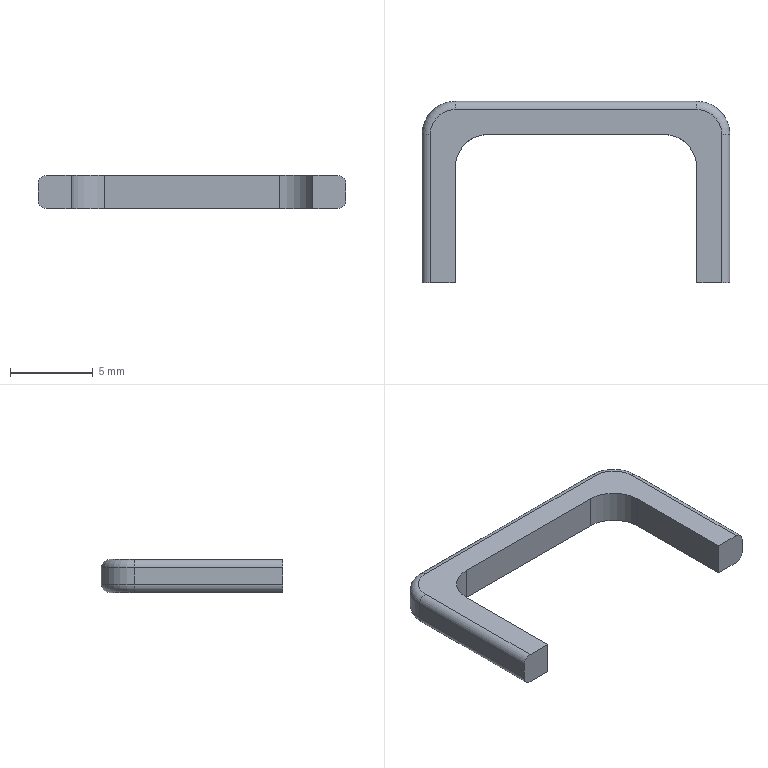Part | SolidWorks | features Fillet 2, ExtruThin 1 | 1 solid | 24 faces | box 18.597 x 10.954 x 2 mm | volume 141.898 mm3 | plane 10 | cylinder 10 | torus 4 | commonest cylinder face diameters 1 x6 4 x4
STEP:
#1=CARTESIAN_POINT('',(-2.,8.954,1.5));
#2=VERTEX_POINT('',#1);
#3=CARTESIAN_POINT('',(-2.,8.954,0.5));
#4=VERTEX_POINT('',#3);
#5=CARTESIAN_POINT('',(-2.,8.954,2.));
#6=DIRECTION('',(0.,0.,-1.));
#7=VECTOR('',#6,1000.);
#8=LINE('',#5,#7);
#9=EDGE_CURVE('',#2,#4,#8,.T.);
#10=ORIENTED_EDGE('',*,*,#9,.T.);
#11=CARTESIAN_POINT('',(-2.,0.,0.5));
#12=VERTEX_POINT('',#11);
#13=CARTESIAN_POINT('',(-2.,0.,0.5));
#14=DIRECTION('',(0.,-1.,0.));
#15=VECTOR('',#14,1000.);
#16=LINE('',#13,#15);
#17=EDGE_CURVE('',#4,#12,#16,.T.);
#18=ORIENTED_EDGE('',*,*,#17,.T.);
#19=CARTESIAN_POINT('',(-2.,0.,1.5));
#20=VERTEX_POINT('',#19);
#21=CARTESIAN_POINT('',(-2.,0.,2.));
#22=DIRECTION('',(0.,0.,-1.));
#23=VECTOR('',#22,1000.);
#24=LINE('',#21,#23);
#25=EDGE_CURVE('',#20,#12,#24,.T.);
#26=ORIENTED_EDGE('',*,*,#25,.F.);
#27=CARTESIAN_POINT('',(-2.,8.954,1.5));
#28=DIRECTION('',(0.,1.,0.));
#29=VECTOR('',#28,1000.);
#30=LINE('',#27,#29);
#31=EDGE_CURVE('',#20,#2,#30,.T.);
#32=ORIENTED_EDGE('',*,*,#31,.T.);
#33=EDGE_LOOP('',(#10,#18,#26,#32));
#34=FACE_OUTER_BOUND('',#33,.T.);
#35=CARTESIAN_POINT('',(-2.,0.,2.));
#36=DIRECTION('',(1.,0.,0.));
#37=DIRECTION('',(0.,0.,-1.));
#38=AXIS2_PLACEMENT_3D('',#35,#36,#37);
#39=PLANE('',#38);
#40=ADVANCED_FACE('',(#34),#39,.F.);
#41=ORIENTED_EDGE('',*,*,#25,.T.);
#42=CARTESIAN_POINT('',(-1.5,0.,0.));
#43=VERTEX_POINT('',#42);
#44=CARTESIAN_POINT('',(-1.5,0.,0.5));
#45=DIRECTION('',(0.,-1.,0.));
#46=DIRECTION('',(0.,0.,-1.));
#47=AXIS2_PLACEMENT_3D('',#44,#45,#46);
#48=CIRCLE('',#47,0.5);
#49=EDGE_CURVE('',#12,#43,#48,.T.);
#50=ORIENTED_EDGE('',*,*,#49,.T.);
#51=CARTESIAN_POINT('',(0.,0.,0.));
#52=VERTEX_POINT('',#51);
#53=CARTESIAN_POINT('',(0.,0.,0.));
#54=DIRECTION('',(-1.,0.,0.));
#55=VECTOR('',#54,1000.);
#56=LINE('',#53,#55);
#57=EDGE_CURVE('',#52,#43,#56,.T.);
#58=ORIENTED_EDGE('',*,*,#57,.F.);
#59=CARTESIAN_POINT('',(0.,0.,2.));
#60=VERTEX_POINT('',#59);
#61=CARTESIAN_POINT('',(0.,0.,2.));
#62=DIRECTION('',(0.,0.,-1.));
#63=VECTOR('',#62,1000.);
#64=LINE('',#61,#63);
#65=EDGE_CURVE('',#60,#52,#64,.T.);
#66=ORIENTED_EDGE('',*,*,#65,.F.);
#67=CARTESIAN_POINT('',(-1.5,0.,2.));
#68=VERTEX_POINT('',#67);
#69=CARTESIAN_POINT('',(0.,0.,2.));
#70=DIRECTION('',(-1.,0.,0.));
#71=VECTOR('',#70,1000.);
#72=LINE('',#69,#71);
#73=EDGE_CURVE('',#60,#68,#72,.T.);
#74=ORIENTED_EDGE('',*,*,#73,.T.);
#75=CARTESIAN_POINT('',(-1.5,0.,1.5));
#76=DIRECTION('',(0.,-1.,0.));
#77=DIRECTION('',(0.,0.,-1.));
#78=AXIS2_PLACEMENT_3D('',#75,#76,#77);
#79=CIRCLE('',#78,0.5);
#80=EDGE_CURVE('',#68,#20,#79,.T.);
#81=ORIENTED_EDGE('',*,*,#80,.T.);
#82=EDGE_LOOP('',(#41,#50,#58,#66,#74,#81));
#83=FACE_OUTER_BOUND('',#82,.T.);
#84=CARTESIAN_POINT('',(0.,0.,2.));
#85=DIRECTION('',(0.,-1.,0.));
#86=DIRECTION('',(0.,0.,-1.));
#87=AXIS2_PLACEMENT_3D('',#84,#85,#86);
#88=PLANE('',#87);
#89=ADVANCED_FACE('',(#83),#88,.T.);
#90=CARTESIAN_POINT('',(0.,6.954,0.));
#91=VERTEX_POINT('',#90);
#92=CARTESIAN_POINT('',(0.,0.,0.));
#93=DIRECTION('',(0.,-1.,0.));
#94=VECTOR('',#93,1000.);
#95=LINE('',#92,#94);
#96=EDGE_CURVE('',#91,#52,#95,.T.);
#97=ORIENTED_EDGE('',*,*,#96,.F.);
#98=CARTESIAN_POINT('',(0.,6.954,2.));
#99=VERTEX_POINT('',#98);
#100=CARTESIAN_POINT('',(0.,6.954,2.));
#101=DIRECTION('',(0.,0.,1.));
#102=VECTOR('',#101,1000.);
#103=LINE('',#100,#102);
#104=EDGE_CURVE('',#91,#99,#103,.T.);
#105=ORIENTED_EDGE('',*,*,#104,.T.);
#106=CARTESIAN_POINT('',(0.,0.,2.));
#107=DIRECTION('',(0.,-1.,0.));
#108=VECTOR('',#107,1000.);
#109=LINE('',#106,#108);
#110=EDGE_CURVE('',#99,#60,#109,.T.);
#111=ORIENTED_EDGE('',*,*,#110,.T.);
#112=ORIENTED_EDGE('',*,*,#65,.T.);
#113=EDGE_LOOP('',(#97,#105,#111,#112));
#114=FACE_OUTER_BOUND('',#113,.T.);
#115=CARTESIAN_POINT('',(0.,0.,2.));
#116=DIRECTION('',(1.,0.,0.));
#117=DIRECTION('',(0.,0.,-1.));
#118=AXIS2_PLACEMENT_3D('',#115,#116,#117);
#119=PLANE('',#118);
#120=ADVANCED_FACE('',(#114),#119,.T.);
#121=CARTESIAN_POINT('',(12.597,8.954,0.));
#122=VERTEX_POINT('',#121);
#123=CARTESIAN_POINT('',(2.,8.954,0.));
#124=VERTEX_POINT('',#123);
#125=CARTESIAN_POINT('',(0.,8.954,0.));
#126=DIRECTION('',(-1.,0.,0.));
#127=VECTOR('',#126,1000.);
#128=LINE('',#125,#127);
#129=EDGE_CURVE('',#122,#124,#128,.T.);
#130=ORIENTED_EDGE('',*,*,#129,.F.);
#131=CARTESIAN_POINT('',(12.597,8.954,2.));
#132=VERTEX_POINT('',#131);
#133=CARTESIAN_POINT('',(12.597,8.954,2.));
#134=DIRECTION('',(0.,0.,1.));
#135=VECTOR('',#134,1000.);
#136=LINE('',#133,#135);
#137=EDGE_CURVE('',#122,#132,#136,.T.);
#138=ORIENTED_EDGE('',*,*,#137,.T.);
#139=CARTESIAN_POINT('',(2.,8.954,2.));
#140=VERTEX_POINT('',#139);
#141=CARTESIAN_POINT('',(0.,8.954,2.));
#142=DIRECTION('',(-1.,0.,0.));
#143=VECTOR('',#142,1000.);
#144=LINE('',#141,#143);
#145=EDGE_CURVE('',#132,#140,#144,.T.);
#146=ORIENTED_EDGE('',*,*,#145,.T.);
#147=CARTESIAN_POINT('',(2.,8.954,0.));
#148=DIRECTION('',(0.,0.,-1.));
#149=VECTOR('',#148,1000.);
#150=LINE('',#147,#149);
#151=EDGE_CURVE('',#140,#124,#150,.T.);
#152=ORIENTED_EDGE('',*,*,#151,.T.);
#153=EDGE_LOOP('',(#130,#138,#146,#152));
#154=FACE_OUTER_BOUND('',#153,.T.);
#155=CARTESIAN_POINT('',(0.,8.954,2.));
#156=DIRECTION('',(0.,-1.,0.));
#157=DIRECTION('',(0.,0.,-1.));
#158=AXIS2_PLACEMENT_3D('',#155,#156,#157);
#159=PLANE('',#158);
#160=ADVANCED_FACE('',(#154),#159,.T.);
#161=CARTESIAN_POINT('',(14.597,0.,2.));
#162=VERTEX_POINT('',#161);
#163=CARTESIAN_POINT('',(14.597,6.954,2.));
#164=VERTEX_POINT('',#163);
#165=CARTESIAN_POINT('',(14.597,0.,2.));
#166=DIRECTION('',(0.,1.,0.));
#167=VECTOR('',#166,1000.);
#168=LINE('',#165,#167);
#169=EDGE_CURVE('',#162,#164,#168,.T.);
#170=ORIENTED_EDGE('',*,*,#169,.T.);
#171=CARTESIAN_POINT('',(14.597,6.954,0.));
#172=VERTEX_POINT('',#171);
#173=CARTESIAN_POINT('',(14.597,6.954,0.));
#174=DIRECTION('',(0.,0.,-1.));
#175=VECTOR('',#174,1000.);
#176=LINE('',#173,#175);
#177=EDGE_CURVE('',#164,#172,#176,.T.);
#178=ORIENTED_EDGE('',*,*,#177,.T.);
#179=CARTESIAN_POINT('',(14.597,0.,0.));
#180=VERTEX_POINT('',#179);
#181=CARTESIAN_POINT('',(14.597,0.,0.));
#182=DIRECTION('',(0.,1.,0.));
#183=VECTOR('',#182,1000.);
#184=LINE('',#181,#183);
#185=EDGE_CURVE('',#180,#172,#184,.T.);
#186=ORIENTED_EDGE('',*,*,#185,.F.);
#187=CARTESIAN_POINT('',(14.597,0.,2.));
#188=DIRECTION('',(0.,0.,-1.));
#189=VECTOR('',#188,1000.);
#190=LINE('',#187,#189);
#191=EDGE_CURVE('',#162,#180,#190,.T.);
#192=ORIENTED_EDGE('',*,*,#191,.F.);
#193=EDGE_LOOP('',(#170,#178,#186,#192));
#194=FACE_OUTER_BOUND('',#193,.T.);
#195=CARTESIAN_POINT('',(14.597,0.,2.));
#196=DIRECTION('',(-1.,0.,0.));
#197=DIRECTION('',(0.,0.,1.));
#198=AXIS2_PLACEMENT_3D('',#195,#196,#197);
#199=PLANE('',#198);
#200=ADVANCED_FACE('',(#194),#199,.T.);
#201=CARTESIAN_POINT('',(16.097,0.,0.));
#202=VERTEX_POINT('',#201);
#203=CARTESIAN_POINT('',(16.597,0.,0.));
#204=DIRECTION('',(-1.,0.,0.));
#205=VECTOR('',#204,1000.);
#206=LINE('',#203,#205);
#207=EDGE_CURVE('',#202,#180,#206,.T.);
#208=ORIENTED_EDGE('',*,*,#207,.F.);
#209=CARTESIAN_POINT('',(16.597,0.,0.5));
#210=VERTEX_POINT('',#209);
#211=CARTESIAN_POINT('',(16.097,0.,0.5));
#212=DIRECTION('',(0.,-1.,0.));
#213=DIRECTION('',(0.,0.,-1.));
#214=AXIS2_PLACEMENT_3D('',#211,#212,#213);
#215=CIRCLE('',#214,0.5);
#216=EDGE_CURVE('',#202,#210,#215,.T.);
#217=ORIENTED_EDGE('',*,*,#216,.T.);
#218=CARTESIAN_POINT('',(16.597,0.,1.5));
#219=VERTEX_POINT('',#218);
#220=CARTESIAN_POINT('',(16.597,0.,2.));
#221=DIRECTION('',(0.,0.,-1.));
#222=VECTOR('',#221,1000.);
#223=LINE('',#220,#222);
#224=EDGE_CURVE('',#219,#210,#223,.T.);
#225=ORIENTED_EDGE('',*,*,#224,.F.);
#226=CARTESIAN_POINT('',(16.097,0.,2.));
#227=VERTEX_POINT('',#226);
#228=CARTESIAN_POINT('',(16.097,0.,1.5));
#229=DIRECTION('',(0.,-1.,0.));
#230=DIRECTION('',(0.,0.,-1.));
#231=AXIS2_PLACEMENT_3D('',#228,#229,#230);
#232=CIRCLE('',#231,0.5);
#233=EDGE_CURVE('',#219,#227,#232,.T.);
#234=ORIENTED_EDGE('',*,*,#233,.T.);
#235=CARTESIAN_POINT('',(16.597,0.,2.));
#236=DIRECTION('',(-1.,0.,0.));
#237=VECTOR('',#236,1000.);
#238=LINE('',#235,#237);
#239=EDGE_CURVE('',#227,#162,#238,.T.);
#240=ORIENTED_EDGE('',*,*,#239,.T.);
#241=ORIENTED_EDGE('',*,*,#191,.T.);
#242=EDGE_LOOP('',(#208,#217,#225,#234,#240,#241));
#243=FACE_OUTER_BOUND('',#242,.T.);
#244=CARTESIAN_POINT('',(16.597,0.,2.));
#245=DIRECTION('',(0.,-1.,0.));
#246=DIRECTION('',(0.,0.,-1.));
#247=AXIS2_PLACEMENT_3D('',#244,#245,#246);
#248=PLANE('',#247);
#249=ADVANCED_FACE('',(#243),#248,.T.);
#250=ORIENTED_EDGE('',*,*,#224,.T.);
#251=CARTESIAN_POINT('',(16.597,8.954,0.5));
#252=VERTEX_POINT('',#251);
#253=CARTESIAN_POINT('',(16.597,0.,0.5));
#254=DIRECTION('',(0.,1.,0.));
#255=VECTOR('',#254,1000.);
#256=LINE('',#253,#255);
#257=EDGE_CURVE('',#210,#252,#256,.T.);
#258=ORIENTED_EDGE('',*,*,#257,.T.);
#259=CARTESIAN_POINT('',(16.597,8.954,1.5));
#260=VERTEX_POINT('',#259);
#261=CARTESIAN_POINT('',(16.597,8.954,2.));
#262=DIRECTION('',(0.,0.,1.));
#263=VECTOR('',#262,1000.);
#264=LINE('',#261,#263);
#265=EDGE_CURVE('',#252,#260,#264,.T.);
#266=ORIENTED_EDGE('',*,*,#265,.T.);
#267=CARTESIAN_POINT('',(16.597,0.,1.5));
#268=DIRECTION('',(0.,-1.,0.));
#269=VECTOR('',#268,1000.);
#270=LINE('',#267,#269);
#271=EDGE_CURVE('',#260,#219,#270,.T.);
#272=ORIENTED_EDGE('',*,*,#271,.T.);
#273=EDGE_LOOP('',(#250,#258,#266,#272));
#274=FACE_OUTER_BOUND('',#273,.T.);
#275=CARTESIAN_POINT('',(16.597,0.,2.));
#276=DIRECTION('',(-1.,0.,0.));
#277=DIRECTION('',(0.,0.,1.));
#278=AXIS2_PLACEMENT_3D('',#275,#276,#277);
#279=PLANE('',#278);
#280=ADVANCED_FACE('',(#274),#279,.F.);
#281=CARTESIAN_POINT('',(14.597,10.954,1.5));
#282=VERTEX_POINT('',#281);
#283=CARTESIAN_POINT('',(14.597,10.954,0.5));
#284=VERTEX_POINT('',#283);
#285=CARTESIAN_POINT('',(14.597,10.954,2.));
#286=DIRECTION('',(0.,0.,-1.));
#287=VECTOR('',#286,1000.);
#288=LINE('',#285,#287);
#289=EDGE_CURVE('',#282,#284,#288,.T.);
#290=ORIENTED_EDGE('',*,*,#289,.T.);
#291=CARTESIAN_POINT('',(0.,10.954,0.5));
#292=VERTEX_POINT('',#291);
#293=CARTESIAN_POINT('',(0.,10.954,0.5));
#294=DIRECTION('',(-1.,0.,0.));
#295=VECTOR('',#294,1000.);
#296=LINE('',#293,#295);
#297=EDGE_CURVE('',#284,#292,#296,.T.);
#298=ORIENTED_EDGE('',*,*,#297,.T.);
#299=CARTESIAN_POINT('',(0.,10.954,1.5));
#300=VERTEX_POINT('',#299);
#301=CARTESIAN_POINT('',(0.,10.954,2.));
#302=DIRECTION('',(0.,0.,1.));
#303=VECTOR('',#302,1000.);
#304=LINE('',#301,#303);
#305=EDGE_CURVE('',#292,#300,#304,.T.);
#306=ORIENTED_EDGE('',*,*,#305,.T.);
#307=CARTESIAN_POINT('',(14.597,10.954,1.5));
#308=DIRECTION('',(1.,0.,0.));
#309=VECTOR('',#308,1000.);
#310=LINE('',#307,#309);
#311=EDGE_CURVE('',#300,#282,#310,.T.);
#312=ORIENTED_EDGE('',*,*,#311,.T.);
#313=EDGE_LOOP('',(#290,#298,#306,#312));
#314=FACE_OUTER_BOUND('',#313,.T.);
#315=CARTESIAN_POINT('',(0.,10.954,2.));
#316=DIRECTION('',(0.,-1.,0.));
#317=DIRECTION('',(0.,0.,-1.));
#318=AXIS2_PLACEMENT_3D('',#315,#316,#317);
#319=PLANE('',#318);
#320=ADVANCED_FACE('',(#314),#319,.F.);
#321=ORIENTED_EDGE('',*,*,#239,.F.);
#322=CARTESIAN_POINT('',(16.097,8.954,2.));
#323=VERTEX_POINT('',#322);
#324=CARTESIAN_POINT('',(16.097,8.954,2.));
#325=DIRECTION('',(0.,1.,0.));
#326=VECTOR('',#325,1000.);
#327=LINE('',#324,#326);
#328=EDGE_CURVE('',#227,#323,#327,.T.);
#329=ORIENTED_EDGE('',*,*,#328,.T.);
#330=CARTESIAN_POINT('',(14.597,10.454,2.));
#331=VERTEX_POINT('',#330);
#332=CARTESIAN_POINT('',(14.597,8.954,2.));
#333=DIRECTION('',(0.,0.,1.));
#334=DIRECTION('',(1.,0.,0.));
#335=AXIS2_PLACEMENT_3D('',#332,#333,#334);
#336=CIRCLE('',#335,1.5);
#337=EDGE_CURVE('',#323,#331,#336,.T.);
#338=ORIENTED_EDGE('',*,*,#337,.T.);
#339=CARTESIAN_POINT('',(0.,10.454,2.));
#340=VERTEX_POINT('',#339);
#341=CARTESIAN_POINT('',(0.,10.454,2.));
#342=DIRECTION('',(-1.,0.,0.));
#343=VECTOR('',#342,1000.);
#344=LINE('',#341,#343);
#345=EDGE_CURVE('',#331,#340,#344,.T.);
#346=ORIENTED_EDGE('',*,*,#345,.T.);
#347=CARTESIAN_POINT('',(-1.5,8.954,2.));
#348=VERTEX_POINT('',#347);
#349=CARTESIAN_POINT('',(0.,8.954,2.));
#350=DIRECTION('',(0.,0.,1.));
#351=DIRECTION('',(1.,0.,0.));
#352=AXIS2_PLACEMENT_3D('',#349,#350,#351);
#353=CIRCLE('',#352,1.5);
#354=EDGE_CURVE('',#340,#348,#353,.T.);
#355=ORIENTED_EDGE('',*,*,#354,.T.);
#356=CARTESIAN_POINT('',(-1.5,0.,2.));
#357=DIRECTION('',(0.,-1.,0.));
#358=VECTOR('',#357,1000.);
#359=LINE('',#356,#358);
#360=EDGE_CURVE('',#348,#68,#359,.T.);
#361=ORIENTED_EDGE('',*,*,#360,.T.);
#362=ORIENTED_EDGE('',*,*,#73,.F.);
#363=ORIENTED_EDGE('',*,*,#110,.F.);
#364=CARTESIAN_POINT('',(2.,6.954,2.));
#365=DIRECTION('',(0.,0.,-1.));
#366=DIRECTION('',(1.,0.,0.));
#367=AXIS2_PLACEMENT_3D('',#364,#365,#366);
#368=CIRCLE('',#367,2.);
#369=EDGE_CURVE('',#99,#140,#368,.T.);
#370=ORIENTED_EDGE('',*,*,#369,.T.);
#371=ORIENTED_EDGE('',*,*,#145,.F.);
#372=CARTESIAN_POINT('',(12.597,6.954,2.));
#373=DIRECTION('',(0.,0.,-1.));
#374=DIRECTION('',(1.,0.,0.));
#375=AXIS2_PLACEMENT_3D('',#372,#373,#374);
#376=CIRCLE('',#375,2.);
#377=EDGE_CURVE('',#132,#164,#376,.T.);
#378=ORIENTED_EDGE('',*,*,#377,.T.);
#379=ORIENTED_EDGE('',*,*,#169,.F.);
#380=EDGE_LOOP('',(#321,#329,#338,#346,#355,#361,#362,#363,#370,#371,#378,#379));
#381=FACE_OUTER_BOUND('',#380,.T.);
#382=CARTESIAN_POINT('',(0.,0.,2.));
#383=DIRECTION('',(0.,0.,1.));
#384=DIRECTION('',(1.,0.,0.));
#385=AXIS2_PLACEMENT_3D('',#382,#383,#384);
#386=PLANE('',#385);
#387=ADVANCED_FACE('',(#381),#386,.T.);
#388=CARTESIAN_POINT('',(14.597,10.454,0.));
#389=VERTEX_POINT('',#388);
#390=CARTESIAN_POINT('',(16.097,8.954,0.));
#391=VERTEX_POINT('',#390);
#392=CARTESIAN_POINT('',(14.597,8.954,0.));
#393=DIRECTION('',(0.,0.,-1.));
#394=DIRECTION('',(1.,0.,0.));
#395=AXIS2_PLACEMENT_3D('',#392,#393,#394);
#396=CIRCLE('',#395,1.5);
#397=EDGE_CURVE('',#389,#391,#396,.T.);
#398=ORIENTED_EDGE('',*,*,#397,.T.);
#399=CARTESIAN_POINT('',(16.097,0.,0.));
#400=DIRECTION('',(0.,-1.,0.));
#401=VECTOR('',#400,1000.);
#402=LINE('',#399,#401);
#403=EDGE_CURVE('',#391,#202,#402,.T.);
#404=ORIENTED_EDGE('',*,*,#403,.T.);
#405=ORIENTED_EDGE('',*,*,#207,.T.);
#406=ORIENTED_EDGE('',*,*,#185,.T.);
#407=CARTESIAN_POINT('',(12.597,6.954,0.));
#408=DIRECTION('',(0.,0.,1.));
#409=DIRECTION('',(1.,0.,0.));
#410=AXIS2_PLACEMENT_3D('',#407,#408,#409);
#411=CIRCLE('',#410,2.);
#412=EDGE_CURVE('',#172,#122,#411,.T.);
#413=ORIENTED_EDGE('',*,*,#412,.T.);
#414=ORIENTED_EDGE('',*,*,#129,.T.);
#415=CARTESIAN_POINT('',(2.,6.954,0.));
#416=DIRECTION('',(0.,0.,1.));
#417=DIRECTION('',(1.,0.,0.));
#418=AXIS2_PLACEMENT_3D('',#415,#416,#417);
#419=CIRCLE('',#418,2.);
#420=EDGE_CURVE('',#124,#91,#419,.T.);
#421=ORIENTED_EDGE('',*,*,#420,.T.);
#422=ORIENTED_EDGE('',*,*,#96,.T.);
#423=ORIENTED_EDGE('',*,*,#57,.T.);
#424=CARTESIAN_POINT('',(-1.5,8.954,0.));
#425=VERTEX_POINT('',#424);
#426=CARTESIAN_POINT('',(-1.5,0.,0.));
#427=DIRECTION('',(0.,1.,0.));
#428=VECTOR('',#427,1000.);
#429=LINE('',#426,#428);
#430=EDGE_CURVE('',#43,#425,#429,.T.);
#431=ORIENTED_EDGE('',*,*,#430,.T.);
#432=CARTESIAN_POINT('',(0.,10.454,0.));
#433=VERTEX_POINT('',#432);
#434=CARTESIAN_POINT('',(0.,8.954,0.));
#435=DIRECTION('',(0.,0.,-1.));
#436=DIRECTION('',(1.,0.,0.));
#437=AXIS2_PLACEMENT_3D('',#434,#435,#436);
#438=CIRCLE('',#437,1.5);
#439=EDGE_CURVE('',#425,#433,#438,.T.);
#440=ORIENTED_EDGE('',*,*,#439,.T.);
#441=CARTESIAN_POINT('',(0.,10.454,0.));
#442=DIRECTION('',(1.,0.,0.));
#443=VECTOR('',#442,1000.);
#444=LINE('',#441,#443);
#445=EDGE_CURVE('',#433,#389,#444,.T.);
#446=ORIENTED_EDGE('',*,*,#445,.T.);
#447=EDGE_LOOP('',(#398,#404,#405,#406,#413,#414,#421,#422,#423,#431,#440,#446));
#448=FACE_OUTER_BOUND('',#447,.T.);
#449=CARTESIAN_POINT('',(0.,0.,0.));
#450=DIRECTION('',(0.,0.,1.));
#451=DIRECTION('',(1.,0.,0.));
#452=AXIS2_PLACEMENT_3D('',#449,#450,#451);
#453=PLANE('',#452);
#454=ADVANCED_FACE('',(#448),#453,.F.);
#455=ORIENTED_EDGE('',*,*,#377,.F.);
#456=ORIENTED_EDGE('',*,*,#137,.F.);
#457=ORIENTED_EDGE('',*,*,#412,.F.);
#458=ORIENTED_EDGE('',*,*,#177,.F.);
#459=EDGE_LOOP('',(#455,#456,#457,#458));
#460=FACE_OUTER_BOUND('',#459,.T.);
#461=CARTESIAN_POINT('',(12.597,6.954,2.));
#462=DIRECTION('',(0.,0.,1.));
#463=DIRECTION('',(1.,0.,0.));
#464=AXIS2_PLACEMENT_3D('',#461,#462,#463);
#465=CYLINDRICAL_SURFACE('',#464,2.);
#466=ADVANCED_FACE('',(#460),#465,.F.);
#467=ORIENTED_EDGE('',*,*,#369,.F.);
#468=ORIENTED_EDGE('',*,*,#104,.F.);
#469=ORIENTED_EDGE('',*,*,#420,.F.);
#470=ORIENTED_EDGE('',*,*,#151,.F.);
#471=EDGE_LOOP('',(#467,#468,#469,#470));
#472=FACE_OUTER_BOUND('',#471,.T.);
#473=CARTESIAN_POINT('',(2.,6.954,2.));
#474=DIRECTION('',(0.,0.,1.));
#475=DIRECTION('',(1.,0.,0.));
#476=AXIS2_PLACEMENT_3D('',#473,#474,#475);
#477=CYLINDRICAL_SURFACE('',#476,2.);
#478=ADVANCED_FACE('',(#472),#477,.F.);
#479=ORIENTED_EDGE('',*,*,#265,.F.);
#480=CARTESIAN_POINT('',(14.597,8.954,0.5));
#481=DIRECTION('',(0.,0.,1.));
#482=DIRECTION('',(1.,0.,0.));
#483=AXIS2_PLACEMENT_3D('',#480,#481,#482);
#484=CIRCLE('',#483,2.);
#485=EDGE_CURVE('',#252,#284,#484,.T.);
#486=ORIENTED_EDGE('',*,*,#485,.T.);
#487=ORIENTED_EDGE('',*,*,#289,.F.);
#488=CARTESIAN_POINT('',(14.597,8.954,1.5));
#489=DIRECTION('',(0.,0.,-1.));
#490=DIRECTION('',(1.,0.,0.));
#491=AXIS2_PLACEMENT_3D('',#488,#489,#490);
#492=CIRCLE('',#491,2.);
#493=EDGE_CURVE('',#282,#260,#492,.T.);
#494=ORIENTED_EDGE('',*,*,#493,.T.);
#495=EDGE_LOOP('',(#479,#486,#487,#494));
#496=FACE_OUTER_BOUND('',#495,.T.);
#497=CARTESIAN_POINT('',(14.597,8.954,2.));
#498=DIRECTION('',(0.,0.,-1.));
#499=DIRECTION('',(-1.,0.,0.));
#500=AXIS2_PLACEMENT_3D('',#497,#498,#499);
#501=CYLINDRICAL_SURFACE('',#500,2.);
#502=ADVANCED_FACE('',(#496),#501,.T.);
#503=ORIENTED_EDGE('',*,*,#305,.F.);
#504=CARTESIAN_POINT('',(0.,8.954,0.5));
#505=DIRECTION('',(0.,0.,1.));
#506=DIRECTION('',(1.,0.,0.));
#507=AXIS2_PLACEMENT_3D('',#504,#505,#506);
#508=CIRCLE('',#507,2.);
#509=EDGE_CURVE('',#292,#4,#508,.T.);
#510=ORIENTED_EDGE('',*,*,#509,.T.);
#511=ORIENTED_EDGE('',*,*,#9,.F.);
#512=CARTESIAN_POINT('',(0.,8.954,1.5));
#513=DIRECTION('',(0.,0.,-1.));
#514=DIRECTION('',(1.,0.,0.));
#515=AXIS2_PLACEMENT_3D('',#512,#513,#514);
#516=CIRCLE('',#515,2.);
#517=EDGE_CURVE('',#2,#300,#516,.T.);
#518=ORIENTED_EDGE('',*,*,#517,.T.);
#519=EDGE_LOOP('',(#503,#510,#511,#518));
#520=FACE_OUTER_BOUND('',#519,.T.);
#521=CARTESIAN_POINT('',(0.,8.954,2.));
#522=DIRECTION('',(0.,0.,-1.));
#523=DIRECTION('',(-1.,0.,0.));
#524=AXIS2_PLACEMENT_3D('',#521,#522,#523);
#525=CYLINDRICAL_SURFACE('',#524,2.);
#526=ADVANCED_FACE('',(#520),#525,.T.);
#527=ORIENTED_EDGE('',*,*,#49,.F.);
#528=ORIENTED_EDGE('',*,*,#17,.F.);
#529=CARTESIAN_POINT('',(-1.5,8.954,0.5));
#530=DIRECTION('',(0.,1.,0.));
#531=DIRECTION('',(0.,0.,1.));
#532=AXIS2_PLACEMENT_3D('',#529,#530,#531);
#533=CIRCLE('',#532,0.5);
#534=EDGE_CURVE('',#425,#4,#533,.T.);
#535=ORIENTED_EDGE('',*,*,#534,.F.);
#536=ORIENTED_EDGE('',*,*,#430,.F.);
#537=EDGE_LOOP('',(#527,#528,#535,#536));
#538=FACE_OUTER_BOUND('',#537,.T.);
#539=CARTESIAN_POINT('',(-1.5,0.,0.5));
#540=DIRECTION('',(0.,-1.,0.));
#541=DIRECTION('',(0.,0.,-1.));
#542=AXIS2_PLACEMENT_3D('',#539,#540,#541);
#543=CYLINDRICAL_SURFACE('',#542,0.5);
#544=ADVANCED_FACE('',(#538),#543,.T.);
#545=ORIENTED_EDGE('',*,*,#534,.T.);
#546=ORIENTED_EDGE('',*,*,#509,.F.);
#547=CARTESIAN_POINT('',(0.,10.454,0.5));
#548=DIRECTION('',(1.,0.,0.));
#549=DIRECTION('',(0.,0.,-1.));
#550=AXIS2_PLACEMENT_3D('',#547,#548,#549);
#551=CIRCLE('',#550,0.5);
#552=EDGE_CURVE('',#433,#292,#551,.T.);
#553=ORIENTED_EDGE('',*,*,#552,.F.);
#554=ORIENTED_EDGE('',*,*,#439,.F.);
#555=EDGE_LOOP('',(#545,#546,#553,#554));
#556=FACE_OUTER_BOUND('',#555,.T.);
#557=CARTESIAN_POINT('',(0.,8.954,0.5));
#558=DIRECTION('',(0.,0.,1.));
#559=DIRECTION('',(1.,0.,0.));
#560=AXIS2_PLACEMENT_3D('',#557,#558,#559);
#561=TOROIDAL_SURFACE('',#560,1.5,0.5);
#562=ADVANCED_FACE('',(#556),#561,.T.);
#563=ORIENTED_EDGE('',*,*,#552,.T.);
#564=ORIENTED_EDGE('',*,*,#297,.F.);
#565=CARTESIAN_POINT('',(14.597,10.454,0.5));
#566=DIRECTION('',(1.,0.,0.));
#567=DIRECTION('',(0.,0.,-1.));
#568=AXIS2_PLACEMENT_3D('',#565,#566,#567);
#569=CIRCLE('',#568,0.5);
#570=EDGE_CURVE('',#389,#284,#569,.T.);
#571=ORIENTED_EDGE('',*,*,#570,.F.);
#572=ORIENTED_EDGE('',*,*,#445,.F.);
#573=EDGE_LOOP('',(#563,#564,#571,#572));
#574=FACE_OUTER_BOUND('',#573,.T.);
#575=CARTESIAN_POINT('',(0.,10.454,0.5));
#576=DIRECTION('',(-1.,0.,0.));
#577=DIRECTION('',(0.,0.,1.));
#578=AXIS2_PLACEMENT_3D('',#575,#576,#577);
#579=CYLINDRICAL_SURFACE('',#578,0.5);
#580=ADVANCED_FACE('',(#574),#579,.T.);
#581=ORIENTED_EDGE('',*,*,#570,.T.);
#582=ORIENTED_EDGE('',*,*,#485,.F.);
#583=CARTESIAN_POINT('',(16.097,8.954,0.5));
#584=DIRECTION('',(0.,-1.,0.));
#585=DIRECTION('',(0.,0.,-1.));
#586=AXIS2_PLACEMENT_3D('',#583,#584,#585);
#587=CIRCLE('',#586,0.5);
#588=EDGE_CURVE('',#391,#252,#587,.T.);
#589=ORIENTED_EDGE('',*,*,#588,.F.);
#590=ORIENTED_EDGE('',*,*,#397,.F.);
#591=EDGE_LOOP('',(#581,#582,#589,#590));
#592=FACE_OUTER_BOUND('',#591,.T.);
#593=CARTESIAN_POINT('',(14.597,8.954,0.5));
#594=DIRECTION('',(0.,0.,1.));
#595=DIRECTION('',(1.,0.,0.));
#596=AXIS2_PLACEMENT_3D('',#593,#594,#595);
#597=TOROIDAL_SURFACE('',#596,1.5,0.5);
#598=ADVANCED_FACE('',(#592),#597,.T.);
#599=ORIENTED_EDGE('',*,*,#216,.F.);
#600=ORIENTED_EDGE('',*,*,#403,.F.);
#601=ORIENTED_EDGE('',*,*,#588,.T.);
#602=ORIENTED_EDGE('',*,*,#257,.F.);
#603=EDGE_LOOP('',(#599,#600,#601,#602));
#604=FACE_OUTER_BOUND('',#603,.T.);
#605=CARTESIAN_POINT('',(16.097,0.,0.5));
#606=DIRECTION('',(0.,1.,0.));
#607=DIRECTION('',(0.,0.,1.));
#608=AXIS2_PLACEMENT_3D('',#605,#606,#607);
#609=CYLINDRICAL_SURFACE('',#608,0.5);
#610=ADVANCED_FACE('',(#604),#609,.T.);
#611=ORIENTED_EDGE('',*,*,#80,.F.);
#612=ORIENTED_EDGE('',*,*,#360,.F.);
#613=CARTESIAN_POINT('',(-1.5,8.954,1.5));
#614=DIRECTION('',(0.,1.,0.));
#615=DIRECTION('',(0.,0.,1.));
#616=AXIS2_PLACEMENT_3D('',#613,#614,#615);
#617=CIRCLE('',#616,0.5);
#618=EDGE_CURVE('',#2,#348,#617,.T.);
#619=ORIENTED_EDGE('',*,*,#618,.F.);
#620=ORIENTED_EDGE('',*,*,#31,.F.);
#621=EDGE_LOOP('',(#611,#612,#619,#620));
#622=FACE_OUTER_BOUND('',#621,.T.);
#623=CARTESIAN_POINT('',(-1.5,0.,1.5));
#624=DIRECTION('',(0.,1.,0.));
#625=DIRECTION('',(0.,0.,1.));
#626=AXIS2_PLACEMENT_3D('',#623,#624,#625);
#627=CYLINDRICAL_SURFACE('',#626,0.5);
#628=ADVANCED_FACE('',(#622),#627,.T.);
#629=ORIENTED_EDGE('',*,*,#618,.T.);
#630=ORIENTED_EDGE('',*,*,#354,.F.);
#631=CARTESIAN_POINT('',(0.,10.454,1.5));
#632=DIRECTION('',(1.,0.,0.));
#633=DIRECTION('',(0.,0.,-1.));
#634=AXIS2_PLACEMENT_3D('',#631,#632,#633);
#635=CIRCLE('',#634,0.5);
#636=EDGE_CURVE('',#300,#340,#635,.T.);
#637=ORIENTED_EDGE('',*,*,#636,.F.);
#638=ORIENTED_EDGE('',*,*,#517,.F.);
#639=EDGE_LOOP('',(#629,#630,#637,#638));
#640=FACE_OUTER_BOUND('',#639,.T.);
#641=CARTESIAN_POINT('',(0.,8.954,1.5));
#642=DIRECTION('',(0.,0.,1.));
#643=DIRECTION('',(1.,0.,0.));
#644=AXIS2_PLACEMENT_3D('',#641,#642,#643);
#645=TOROIDAL_SURFACE('',#644,1.5,0.5);
#646=ADVANCED_FACE('',(#640),#645,.T.);
#647=ORIENTED_EDGE('',*,*,#636,.T.);
#648=ORIENTED_EDGE('',*,*,#345,.F.);
#649=CARTESIAN_POINT('',(14.597,10.454,1.5));
#650=DIRECTION('',(1.,0.,0.));
#651=DIRECTION('',(0.,0.,-1.));
#652=AXIS2_PLACEMENT_3D('',#649,#650,#651);
#653=CIRCLE('',#652,0.5);
#654=EDGE_CURVE('',#282,#331,#653,.T.);
#655=ORIENTED_EDGE('',*,*,#654,.F.);
#656=ORIENTED_EDGE('',*,*,#311,.F.);
#657=EDGE_LOOP('',(#647,#648,#655,#656));
#658=FACE_OUTER_BOUND('',#657,.T.);
#659=CARTESIAN_POINT('',(0.,10.454,1.5));
#660=DIRECTION('',(1.,0.,0.));
#661=DIRECTION('',(0.,0.,-1.));
#662=AXIS2_PLACEMENT_3D('',#659,#660,#661);
#663=CYLINDRICAL_SURFACE('',#662,0.5);
#664=ADVANCED_FACE('',(#658),#663,.T.);
#665=ORIENTED_EDGE('',*,*,#654,.T.);
#666=ORIENTED_EDGE('',*,*,#337,.F.);
#667=CARTESIAN_POINT('',(16.097,8.954,1.5));
#668=DIRECTION('',(0.,-1.,0.));
#669=DIRECTION('',(0.,0.,-1.));
#670=AXIS2_PLACEMENT_3D('',#667,#668,#669);
#671=CIRCLE('',#670,0.5);
#672=EDGE_CURVE('',#260,#323,#671,.T.);
#673=ORIENTED_EDGE('',*,*,#672,.F.);
#674=ORIENTED_EDGE('',*,*,#493,.F.);
#675=EDGE_LOOP('',(#665,#666,#673,#674));
#676=FACE_OUTER_BOUND('',#675,.T.);
#677=CARTESIAN_POINT('',(14.597,8.954,1.5));
#678=DIRECTION('',(0.,0.,1.));
#679=DIRECTION('',(1.,0.,0.));
#680=AXIS2_PLACEMENT_3D('',#677,#678,#679);
#681=TOROIDAL_SURFACE('',#680,1.5,0.5);
#682=ADVANCED_FACE('',(#676),#681,.T.);
#683=ORIENTED_EDGE('',*,*,#233,.F.);
#684=ORIENTED_EDGE('',*,*,#271,.F.);
#685=ORIENTED_EDGE('',*,*,#672,.T.);
#686=ORIENTED_EDGE('',*,*,#328,.F.);
#687=EDGE_LOOP('',(#683,#684,#685,#686));
#688=FACE_OUTER_BOUND('',#687,.T.);
#689=CARTESIAN_POINT('',(16.097,0.,1.5));
#690=DIRECTION('',(0.,-1.,0.));
#691=DIRECTION('',(0.,0.,-1.));
#692=AXIS2_PLACEMENT_3D('',#689,#690,#691);
#693=CYLINDRICAL_SURFACE('',#692,0.5);
#694=ADVANCED_FACE('',(#688),#693,.T.);
#695=CLOSED_SHELL('',(#40,#89,#120,#160,#200,#249,#280,#320,#387,#454,#466,#478,#502,#526,#544,#562,#580,#598,#610,#628,#646,#664,#682,#694));
#696=MANIFOLD_SOLID_BREP('',#695);
#697=CARTESIAN_POINT('',(0.,0.,0.));
#698=DIRECTION('',(0.,0.,1.));
#699=DIRECTION('',(1.,0.,0.));
#700=AXIS2_PLACEMENT_3D('',#697,#698,#699);
#701=(LENGTH_UNIT()NAMED_UNIT(*)SI_UNIT(.MILLI.,.METRE.));
#702=UNCERTAINTY_MEASURE_WITH_UNIT(LENGTH_MEASURE(0.00001),#701,'','');
#703=(NAMED_UNIT(*)PLANE_ANGLE_UNIT()SI_UNIT($,.RADIAN.));
#704=(NAMED_UNIT(*)SI_UNIT($,.STERADIAN.)SOLID_ANGLE_UNIT());
#705=(GEOMETRIC_REPRESENTATION_CONTEXT(3)GLOBAL_UNCERTAINTY_ASSIGNED_CONTEXT((#702))GLOBAL_UNIT_ASSIGNED_CONTEXT((#701,#703,#704))REPRESENTATION_CONTEXT('',''));
#706=ADVANCED_BREP_SHAPE_REPRESENTATION('',(#696,#700),#705);